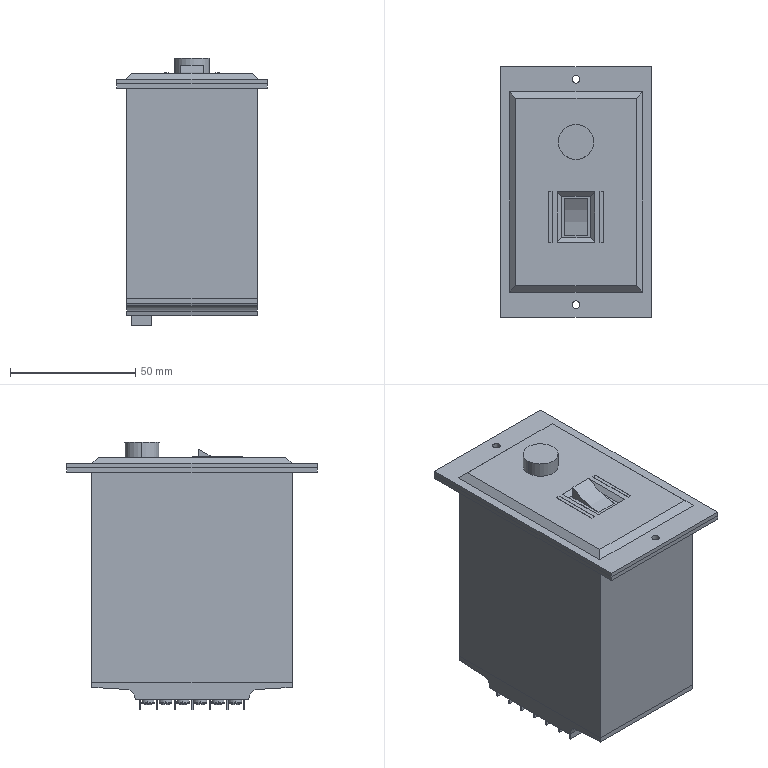Part | SolidWorks | features BaseBody 3 | 3 solids | 221 faces | box 60 x 100 x 107 mm | volume 402424 mm3 | plane 164 | cylinder 33 | spline 24 | commonest cylinder face diameters 5 x16 3 x12 6 x2 14 x2 50 x1